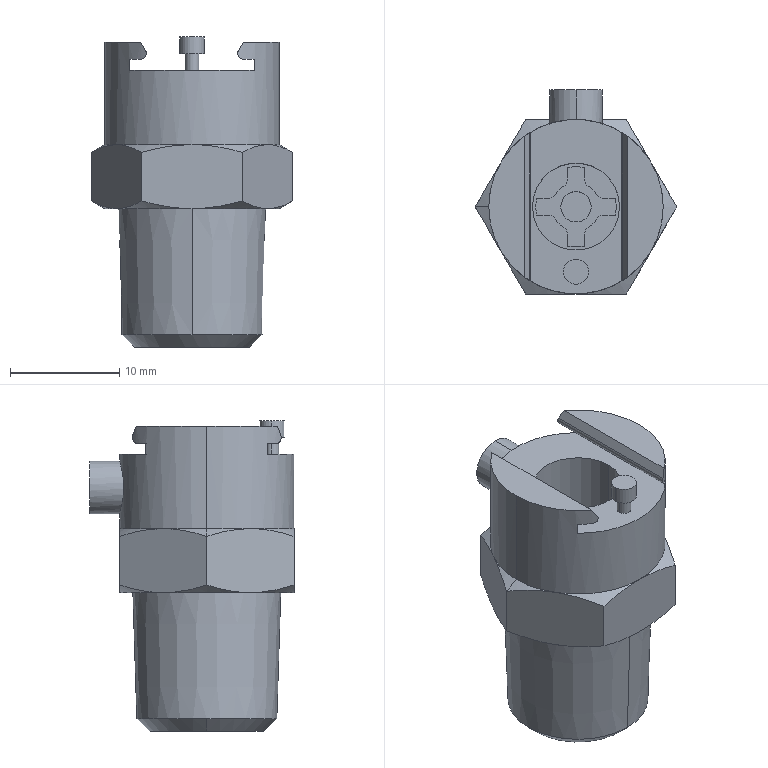Part | SolidWorks | features BaseBody 1 | 1 solid | 98 faces | box 18.478 x 18.72 x 28.448 mm | volume 3801 mm3 | cylinder 39 | plane 33 | cone 22 | spline 4 | commonest cylinder face diameters 1.524 x8 4.42 x8 7.366 x5 1.016 x2 1.27 x2 2.286 x2